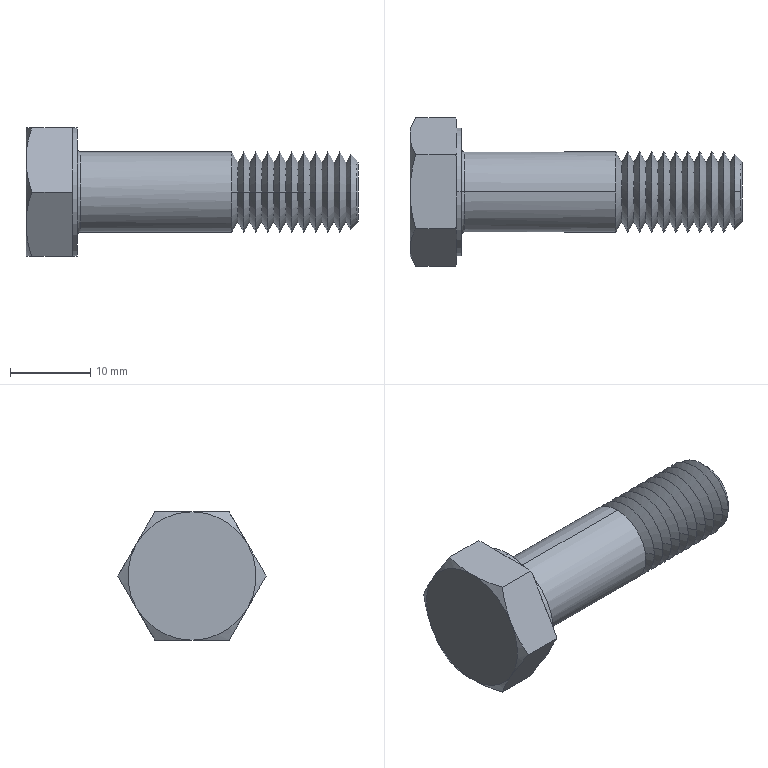Part | SolidWorks | features RevCut 4, Chamfer 1, Extrusion 1, Fillet 1, LPattern 1, Revolution 1 | 1 solid | 95 faces | box 41.4 x 18.475 x 16 mm | volume 3853 mm3 | cone 56 | cylinder 22 | plane 15 | torus 2 | commonest cylinder face diameters 10 x20 16 x2